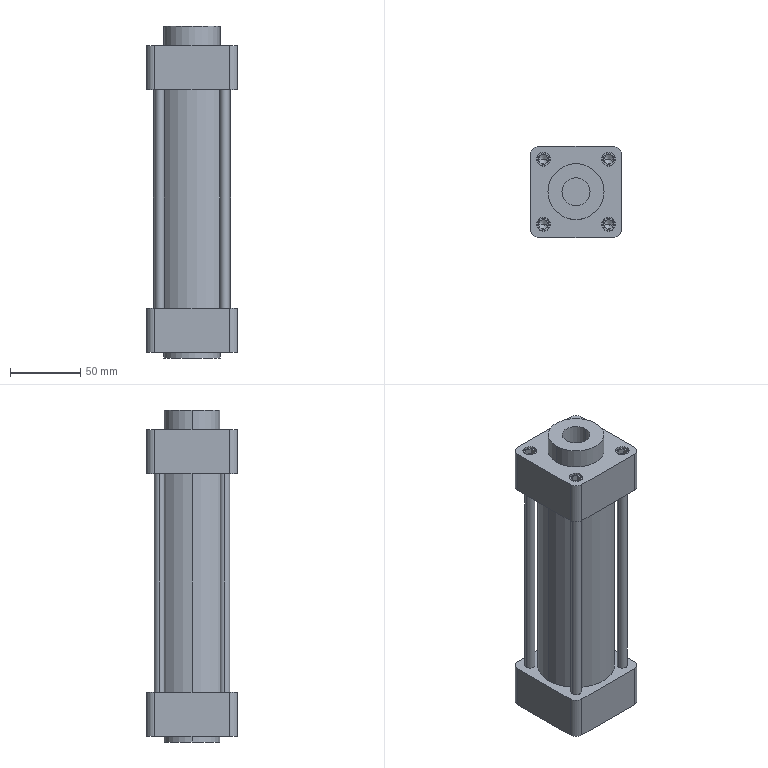Part | STEP file | 1 solid | 196 faces | box 65 x 65 x 237 mm | volume 394428 mm3 | plane 90 | cylinder 82 | cone 24 | commonest cylinder face diameters 6.647 x16 9 x16 10 x16 7.2 x8 12 x8 7.8 x4